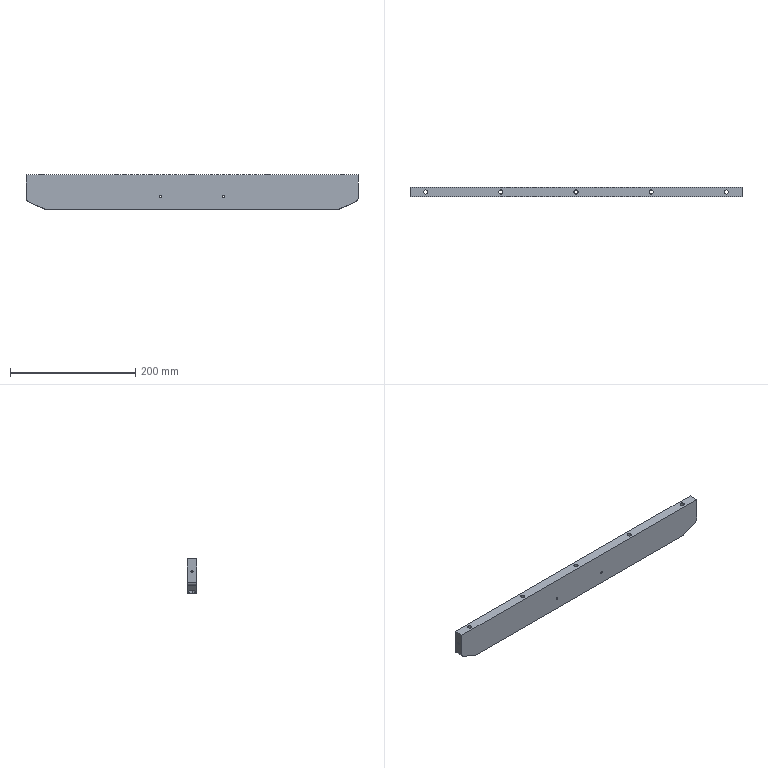Part | SolidWorks | features BaseBody 1 | 1 solid | 73 faces | box 530 x 15 x 55 mm | volume 415651 mm3 | cylinder 44 | cone 16 | plane 13 | commonest cylinder face diameters 3.3 x16 6.6 x10 11 x10 5 x4 10 x4